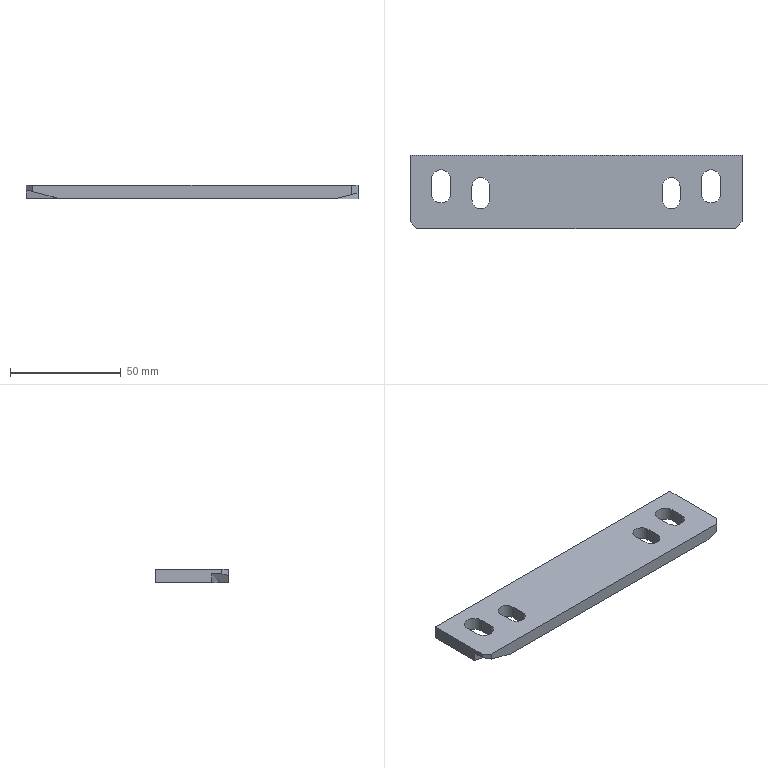Part | STEP file | gslz 2016.10.28-13_id1574_x_t | 1 solid | 29 faces | box 150 x 33 x 6 mm | volume 26801 mm3 | plane 21 | cylinder 8 | commonest cylinder face diameters 8 x4 9 x4